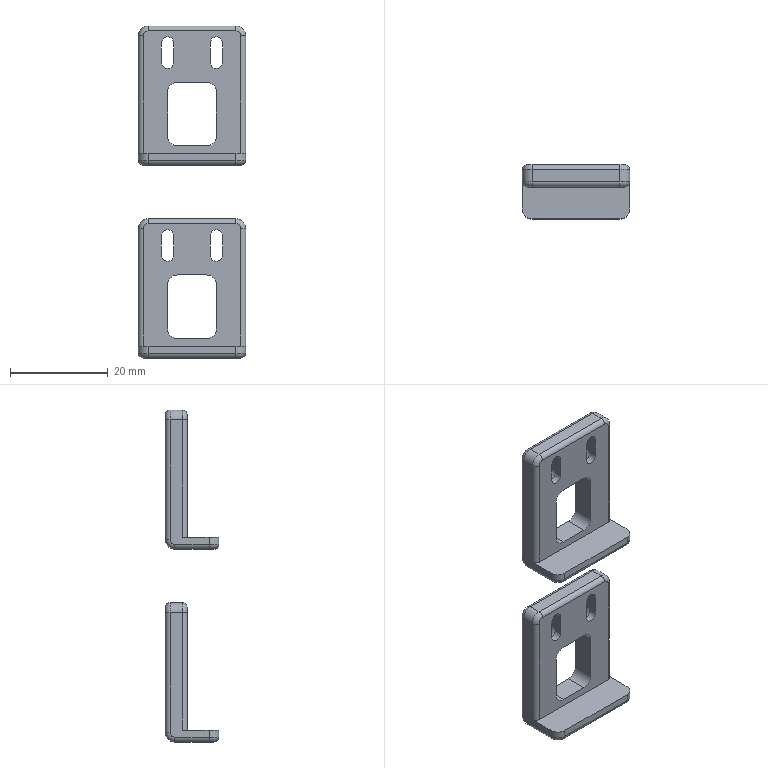CAM job | NX | 3+2 milling | part box 22 x 11 x 68 mm | stock box 25 x 15 x 73 mm
Tools:
number,name,description,diameter,corner_radius,flute_length,length,flutes
17,D2,平底铣刀-粗,2.0,0.0,50.0,75.0,2
3,D3,平底铣刀-粗,3.0,0.0,20.0,75.0,2
6,D6,平底铣刀-粗,6.0,0.0,25.0,75.0,2
9,D10,平底铣刀-粗,10.0,0.0,35.0,75.0,2
11,D4-J,平底铣刀-精,4.0,0.0,50.0,75.0,2
10,D10-J,平底铣刀-精,10.0,0.0,35.0,75.0,2
18,D4R0.5,圆鼻刀-粗,4.0,0.5,50.0,75.0,2
1,D80R0.8飞刀,圆鼻刀-粗,80.0,0.8,50.0,75.0,2
1,D80R0.8飞刀-J,圆鼻刀-精,80.0,0.8,50.0,75.0,2
2,D6倒角刀,倒角刀,6.0,0.0,3.0,25.0,2
Operations:
program,operation,operation_type,tool,method,geometry_group,spindle_rpm,surface_speed,feed_per_tooth,feed_cut,feed_plunge,cut_length_mm,path_length_mm,cut_time_min,machine_time_min
B,底壁铣飞面一刀开粗_COPY,VolumeBased25DMillingOperation,D80R0.8飞刀,分层开粗-切深K-步距G,W-B,2800.0,703.696,0.5357,3000.0,100.0,1409.552,2782.697,0.4699,0.6072
B,底壁铣飞面一刀精光_COPY,VolumeBased25DMillingOperation,D80R0.8飞刀-J,侧刃精光-切深K-步距G,W-B,4000.0,1005.28,0.125,1000.0,100.0,175.998,211.998,0.176,0.1796
B,底壁铣分层开粗-中_COPY,VolumeBased25DMillingOperation,D10,分层开粗-切深K-步距G,W-B,8000.0,251.32,0.25,4000.0,100.0,4200.825,4559.124,1.05,1.086
B,等高精光往复爬面_COPY_COPY_1,ZLevelMilling,D4R0.5,等高爬面-切深K-步距G,W-B,8000.0,100.531,0.2812,4500.0,100.0,1326.699,1521.496,0.2948,0.3143
B,等高精光往复爬面_COPY_COPY_1_COPY,ZLevelMilling,D4R0.5,等高爬面-切深K-步距G,W-B,8000.0,100.531,0.2812,4500.0,100.0,939.921,1041.27,0.2089,0.219
B,等高精光往复爬面_COPY_COPY_1_COPY_COPY,ZLevelMilling,D4R0.5,等高爬面-切深K-步距G,W-B,8000.0,100.531,0.2812,4500.0,100.0,3467.624,3599.962,0.7706,0.7838
B,平面去毛刺6X45L_COPY,SurfaceContour,D6倒角刀,爬面_倒角-切深0-步距G,W-B,6500.0,122.519,0.1154,1500.0,100.0,175.36,538.545,0.1169,0.1532
B,底壁铣精光底面-中_COPY,VolumeBased25DMillingOperation,D10-J,精光步距切深关,W-B,8000.0,251.32,0.0625,1000.0,100.0,208.272,245.271,0.2083,0.212
B,底壁铣精光底面-中_COPY_COPY,VolumeBased25DMillingOperation,D10-J,精光步距切深关,W-B,8000.0,251.32,0.0625,1000.0,100.0,208.271,245.271,0.2083,0.212
B,底壁铣精光侧面-中-选底面_COPY,VolumeBased25DMillingOperation,D10-J,侧刃精光-切深K-步距G,W-B,8000.0,251.32,0.0625,1000.0,100.0,38.683,76.683,0.0387,0.0425
B,底壁铣精光侧面-中-选底面_COPY_COPY,VolumeBased25DMillingOperation,D10-J,侧刃精光-切深K-步距G,W-B,8000.0,251.32,0.0625,1000.0,100.0,38.683,76.683,0.0387,0.0425
A,顶面,FaceMilling,D80R0.8飞刀,侧刃精光-切深K-步距G,W-A,4000.0,1005.31,0.125,1000.0,100.0,162.0,198.0,0.162,0.1656
A,外形粗_2,VolumeBased25DMillingOperation,D10,METHOD,W-A,8000.0,251.327,0.3125,5000.0,80.0,4178.978,4317.881,0.8358,0.8497
A,腰槽粗_1,VolumeBased25DMillingOperation,D6,METHOD,W-A,6000.0,113.0,0.2083,2500.0,100.0,642.101,768.101,0.2568,0.2694
A,底壁铣螺旋开粗-小_COPY,VolumeBased25DMillingOperation,D3,分层开粗-切深K-步距G,W-A,8000.0,75.396,0.125,2000.0,100.0,1369.644,1593.157,0.6848,0.7072
A,腰槽精,VolumeBased25DMillingOperation,D3,METHOD,W-A,6000.0,113.0,0.0417,500.0,100.0,53.48,295.651,0.107,0.1312
A,底壁铣螺旋精光-小_COPY,VolumeBased25DMillingOperation,D3,螺旋精光-切深K-步距G,W-A,8000.0,75.396,0.0375,600.0,100.0,223.332,450.359,0.3722,0.3949
A,腰槽粗_2,VolumeBased25DMillingOperation,D2,METHOD,W-A,6000.0,37.699,0.05,600.0,100.0,1186.451,1433.075,1.977,2.002
A,腰槽精_4,VolumeBased25DMillingOperation,D2,METHOD,W-A,6000.0,37.699,0.0417,500.0,100.0,94.393,366.418,0.1888,0.216
A,清角D4,ZLevelMilling,D4-J,METHOD,W-A,6000.0,75.0,0.25,2500.0,80.0,683.306,804.317,0.2735,0.2856
A,等高精光往复爬面_COPY,ZLevelMilling,D4R0.5,等高爬面-切深K-步距G,W-A,8000.0,100.531,0.2812,4500.0,100.0,2409.926,2494.402,0.5355,0.544
A,等高精光往复爬面_COPY_COPY,ZLevelMilling,D4R0.5,等高爬面-切深K-步距G,W-A,8000.0,100.531,0.2812,4500.0,100.0,3706.401,3799.433,0.8236,0.8329
A,仅选体,SurfaceContour,D6倒角刀,METHOD,W-A,8000.0,150.796,0.1875,3000.0,100.0,175.487,405.837,0.0585,0.0815
A,底壁铣精光侧面-中_COPY,VolumeBased25DMillingOperation,D4-J,侧刃精光-切深K-步距G,W-A,8000.0,100.528,0.05,800.0,100.0,71.57,166.07,0.0895,0.0989
A,外形半精_2,VolumeBased25DMillingOperation,D10-J,METHOD,W-A,8000.0,251.327,0.0625,1000.0,100.0,269.748,466.055,0.2697,0.2894